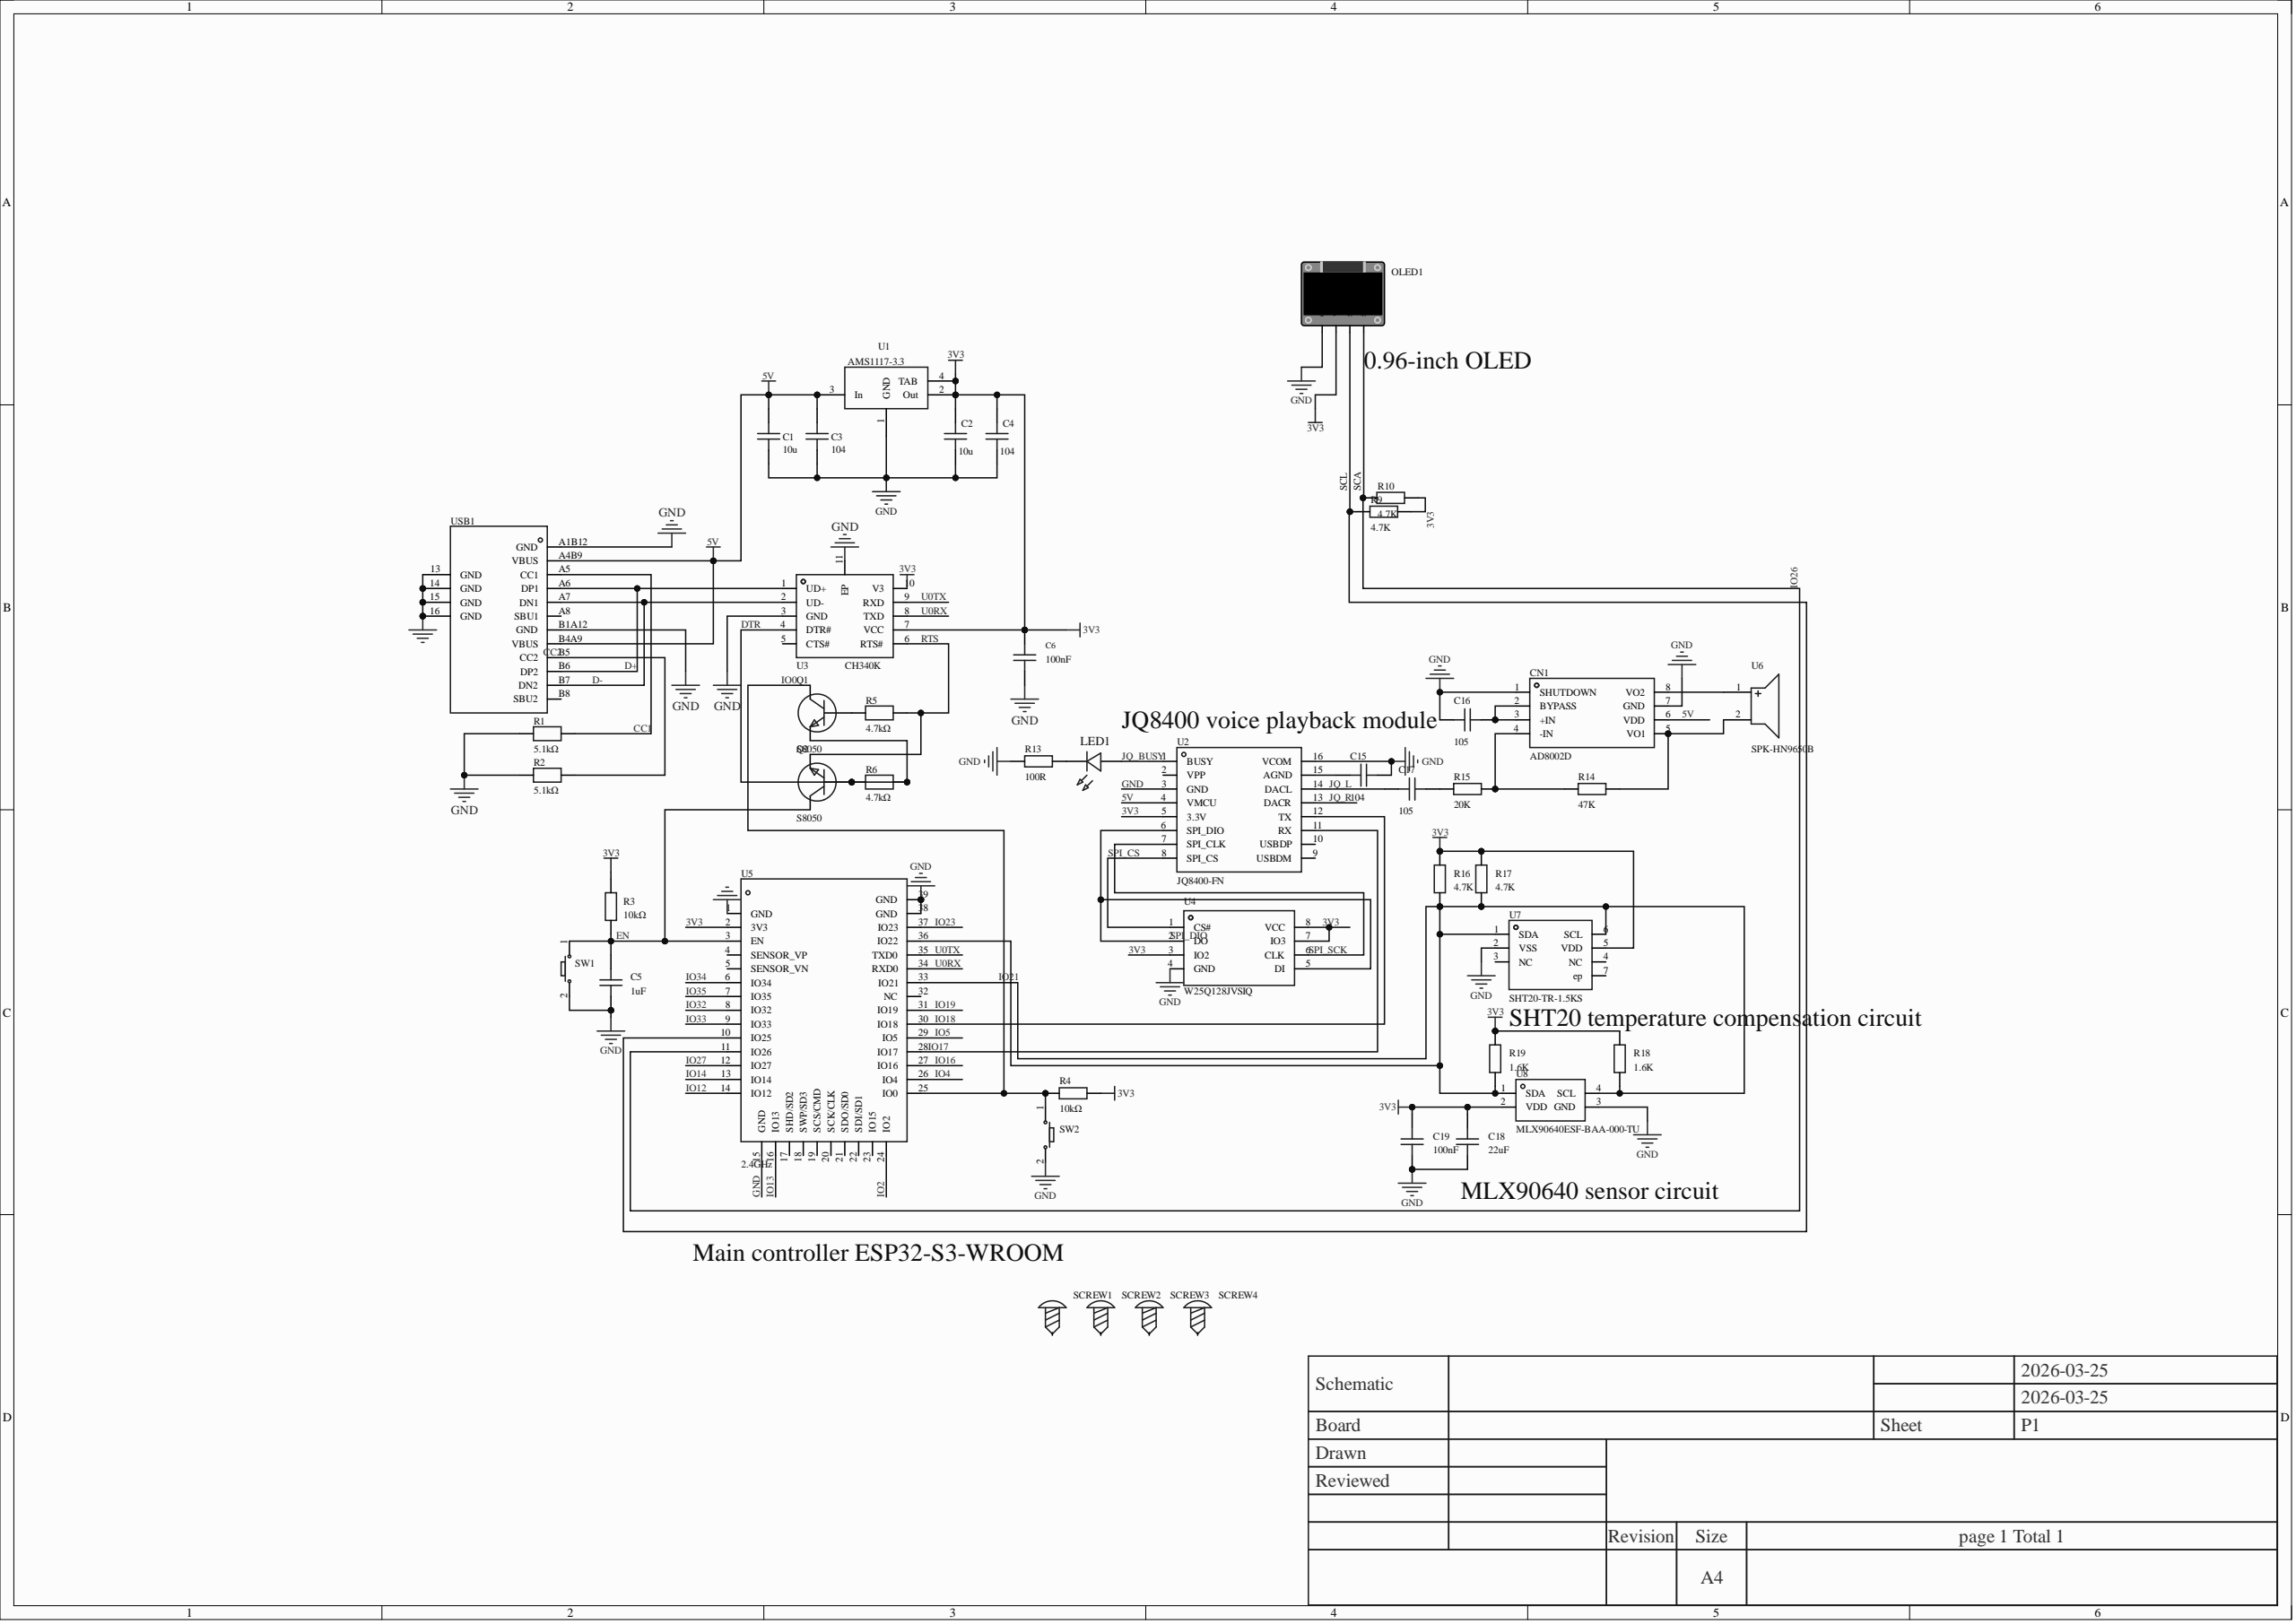Circuit board | Altium Designer | 46 parts | 31 nets
Bill of materials:
Comment,Description,Designator,Footprint,LibRef,Quantity
"10u","","C1, C2","C0805","10u","2"
"104","","C3, C4, C15","C0805","104","3"
"1uF","","C5","C0603","104","1"
"100nF","Capacitance: 100nF; Tolerance: ±10%; Rated voltage: 50V; Dielectric (temperature coefficient): X7R;","C6","C0603_1","GRM155R71H104KE14D","1"
"105","","C16, C17","C0805","104","2"
"22uF","","C18","C0805_1","CAP_0805","1"
"100nF","","C19","C0805_1","CAP_0805","1"
"AD8002D","","CN1","SOP-8_L5.0-W3.8-P1.27-LS6.0-BL","AD8002D","1"
"","","LED1","LED_0603","LED_0603-R","1"
"","","OLED1","0.96OLED_4P","0.96OLED模块_4P","1"
"S8050","","Q1, Q2","SOT-23","S8050","2"
"5.1kΩ","Resistor type: thin-film resistor; Resistance: 5.1kΩ; Tolerance: ±0.1%; Power: 166.667mW;","R1, R2","R0603","TC0350B5101T5E","2"
"10kΩ","Resistor type: thick-film resistor; Resistance: 10kΩ; Tolerance: ±1%; Power: 100mW; Max working voltage: 75V; Temperature coefficient: ±100ppm/?;","R3, R4","R0603","0603WAF1002T5E","2"
"4.7kΩ","Resistor type: thin-film resistor; Resistance: 5.1kΩ; Tolerance: ±0.1%; Power: 166.667mW;","R5, R6","R0603","TC0350B5101T5E","2"
"4.7K","","R9, R10","R0805","Res_0805","2"
"100R","","R13","R0603","Res_0603","1"
"47K","","R14","R0603","Res_0603","1"
"20K","","R15","R0603","Res_0603","1"
"4.7K","","R16, R17","R0603","Res_0603","2"
"1.6K","","R18, R19","R0603","Res_0603","2"
"","","SCREW1, SCREW2, SCREW3, SCREW4","M3螺丝","M3螺丝","4"
"","","SW1, SW2","Key_SMD_3x4x2","Key_SMD_3x4x2","2"
"AMS1117-3.3","","U1","SOT-223_L6.5-W3.5-P2.30-LS7.0-BR","AMS1117-3.3","1"
"JQ8400-FN","","U2","SOP-16_L9.9-W3.9-P1.27-LS6.0-BL","JQ8400-FN","1"
"CH340K","Application function: -; Interface protocol: -;","U3","ESOP-10_L4.9-W3.9-P1.00-LS6.2-BL-EP","CH340K","1"
"W25Q128JVSIQ","Interface type: SPI; Storage capacity: 128Mbit; Clock frequency (fc): 133MHz;","U4","SOIC-8_L5.3-W5.3-P1.27-LS8.0-BL","W25Q128JVSIQ","1"
"2.4GHz","","U5","WIFIM-SMD_ESP32-WROOM-32-N4","ESP32-WROOM-32 (16MB)","1"
"SPK-HN9650B","","U6","BUZ-SMD_L9.6-W9.6-LS10.0-R","SPK-HN9650B","1"
"SHT20-TR-1.5KS","Interface type: I2C;","U7","DFN-6_L3.0-W3.0-P0.95-TR-EP","SHT20-TR-1.5KS","1"
"MLX90640ESF-BAA-000-TU","","U8","TO-39_4P-BD9.3_MLX90640ESF-BAA-000-TU_H5.7","MLX90640ESF-BAA-000-TU_C17380659","1"
"","","USB1","USB-C-SMD_TYPEC-304-BCP16","typec-304-bcp16","1"
Netlist (Protel format):
[
C1
C0805
10u



]
[
C2
C0805
10u



]
[
C3
C0805
104



]
[
C4
C0805
104



]
[
C5
C0603
1uF



]
[
C6
C0603_1
100nF



]
[
C15
C0805
104



]
[
C16
C0805
105



]
[
C17
C0805
105



]
[
C18
C0805_1
22uF



]
[
C19
C0805_1
100nF



]
[
CN1
SOP-8_L5.0-W3.8-P1.27-LS6.0-BL
AD8002D



]
[
LED1
LED_0603




]
[
OLED1
0.96OLED_4P




]
[
Q1
SOT-23
S8050



]
[
Q2
SOT-23
S8050



]
[
R1
R0603
5.1kΩ



]
[
R2
R0603
5.1kΩ



]
[
R3
R0603
10kΩ



]
[
R4
R0603
10kΩ



]
[
R5
R0603
4.7kΩ



]
[
R6
R0603
4.7kΩ



]
[
R9
R0805
4.7K



]
[
R10
R0805
4.7K



]
[
R13
R0603
100R



]
[
R14
R0603
47K



]
[
R15
R0603
20K



]
[
R16
R0603
4.7K



]
[
R17
R0603
4.7K



]
[
R18
R0603
1.6K



]
[
R19
R0603
1.6K



]
[
SCREW1
M3螺丝




]
[
SCREW2
M3螺丝




]
[
SCREW3
M3螺丝




]
[
SCREW4
M3螺丝




]
[
SW1
Key_SMD_3x4x2




]
[
SW2
Key_SMD_3x4x2




]
[
U1
SOT-223_L6.5-W3.5-P2.30-LS7.0-BR
AMS1117-3.3



]
[
U2
SOP-16_L9.9-W3.9-P1.27-LS6.0-BL
JQ8400-FN



]
[
U3
ESOP-10_L4.9-W3.9-P1.00-LS6.2-BL-EP
CH340K



]
[
U4
SOIC-8_L5.3-W5.3-P1.27-LS8.0-BL
W25Q128JVSIQ



]
[
U5
WIFIM-SMD_ESP32-WROOM-32-N4
2.4GHz



]
[
U6
BUZ-SMD_L9.6-W9.6-LS10.0-R
SPK-HN9650B



]
[
U7
DFN-6_L3.0-W3.0-P0.95-TR-EP
SHT20-TR-1.5KS



]
[
U8
TO-39_4P-BD9.3_MLX90640ESF-BAA-000-TU_H5.7
MLX90640ESF-BAA-000-TU



]
[
USB1
USB-C-SMD_TYPEC-304-BCP16




]
(
U0TX
U3-9
U5-35
)
(
U0RX
U3-8
U5-34
)
(
SPI_SCK
U2-7
U4-6
)
(
SPI_DIO
U2-6
U4-2
U4-5
)
(
SPI_CS
U2-8
U4-1
)
(
RTS
Q2-2
R5-1
U3-6
)
(
NetQ1_1
Q1-1
R5-2
)
(
NetOLED1_3
OLED1-3
R9-2
U5-10
)
(
NetLED1_1
LED1-1
R13-2
)
(
NetCN1_8
CN1-8
U6-1
)
(
NetCN1_5
CN1-5
R14-2
U6-2
)
(
NetCN1_4
CN1-4
R14-1
R15-2
)
(
NetC17_1
C17-1
R15-1
)
(
NetC16_1
C16-1
CN1-2
CN1-3
)
(
NetC15_2
C15-2
U2-15
)
(
JQ_L
C17-2
U2-14
)
(
JQ_BUSY
LED1-2
U2-1
)
(
IO26
OLED1-4
R10-2
U5-11
)
(
IO21
R16-1
R17-1
R18-1
R19-1
U5-33
U5-36
U7-1
U7-6
U8-1
U8-4
)
(
IO18
U2-12
U5-30
)
(
IO17
U2-11
U5-28
)
(
IO0
Q1-3
R4-1
SW2-1
U5-25
)
(
GND
C1-1
C2-1
C3-1
C4-1
C5-2
C6-1
C15-1
C16-2
C18-1
C19-1
CN1-1
CN1-7
OLED1-1
R1-2
R2-2
R13-1
SW1-2
SW2-2
U1-1
U2-3
U2-16
U3-3
U3-11
U4-4
U5-1
U5-15
U5-38
U5-39
U7-2
U8-3
USB1-13
USB1-14
USB1-15
USB1-16
USB1-A1B12
USB1-B1A12
)
(
EN
C5-1
Q2-3
R3-1
SW1-1
U5-3
)
(
DTR
Q1-2
Q2-1
R6-1
R6-2
U3-4
)
(
D-
U3-2
USB1-A7
USB1-B7
)
(
D+
U3-1
USB1-A6
USB1-B6
)
(
CC2
R2-1
USB1-B5
)
(
CC1
R1-1
USB1-A5
)
(
5V
C1-2
C3-2
CN1-6
U1-3
U2-4
USB1-A4B9
USB1-B4A9
)
(
3V3
C2-2
C4-2
C6-2
C18-2
C19-2
OLED1-2
R3-2
R4-2
R9-1
R10-1
R16-2
R17-2
R18-2
R19-2
U1-2
U1-4
U2-5
U3-7
U3-10
U4-3
U4-7
U4-8
U5-2
U7-5
U8-2
)